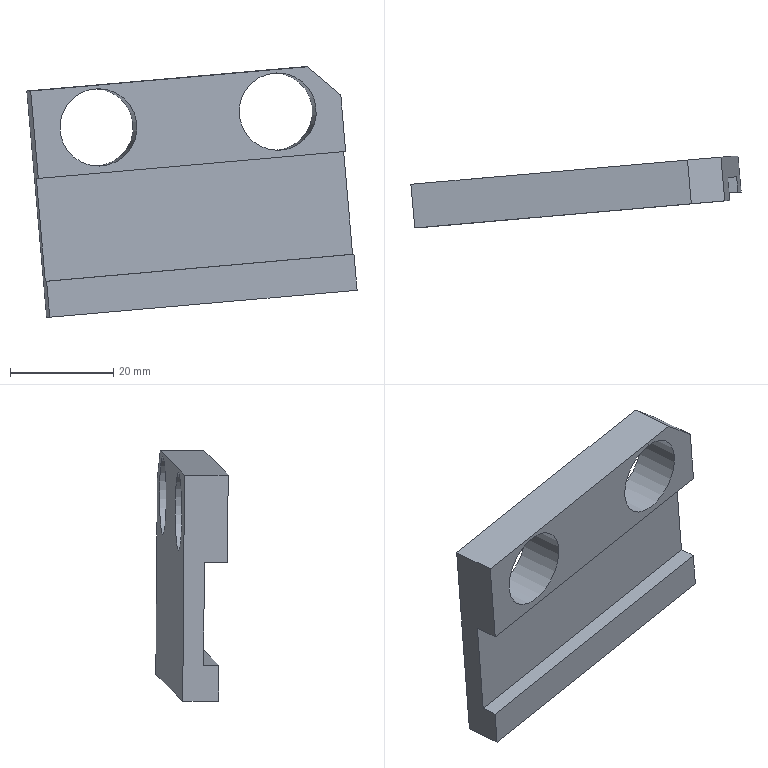Part | NX | features solid 2 | 1 solid | 13 faces | box 63.975 x 14.011 x 48.539 mm | volume 13253 mm3 | plane 11 | cylinder 2 | commonest cylinder face diameters 15 x2
STEP:
#1=CARTESIAN_POINT('',(-431.511,36.53,151.87));
#2=VERTEX_POINT('',#1);
#3=CARTESIAN_POINT('',(-436.313,36.11,146.125));
#4=DIRECTION('',(-0.08716,0.9962,0.));
#5=DIRECTION('',(0.6403,0.05602,0.766));
#6=AXIS2_PLACEMENT_3D('',#3,#4,#5);
#7=CIRCLE('',#6,7.5);
#8=EDGE_CURVE('',#2,#2,#7,.F.);
#9=ORIENTED_EDGE('',*,*,#8,.T.);
#10=EDGE_LOOP('',(#9));
#11=FACE_BOUND('',#10,.T.);
#12=CARTESIAN_POINT('',(-449.432,34.962,153.171));
#13=VERTEX_POINT('',#12);
#14=CARTESIAN_POINT('',(-395.842,39.651,157.877));
#15=VERTEX_POINT('',#14);
#16=CARTESIAN_POINT('',(-433.107,36.391,154.604));
#17=DIRECTION('',(0.9924,0.08682,0.08716));
#18=VECTOR('',#17,1000.);
#19=LINE('',#16,#18);
#20=EDGE_CURVE('',#13,#15,#19,.T.);
#21=ORIENTED_EDGE('',*,*,#20,.T.);
#22=CARTESIAN_POINT('',(-389.367,40.217,152.423));
#23=VERTEX_POINT('',#22);
#24=CARTESIAN_POINT('',(-394.52,39.767,156.764));
#25=DIRECTION('',(-0.7631,-0.06677,0.6428));
#26=VECTOR('',#25,1000.);
#27=LINE('',#24,#26);
#28=EDGE_CURVE('',#15,#23,#27,.F.);
#29=ORIENTED_EDGE('',*,*,#28,.T.);
#30=CARTESIAN_POINT('',(-386.068,40.506,114.567));
#31=VERTEX_POINT('',#30);
#32=CARTESIAN_POINT('',(-389.888,40.172,158.4));
#33=DIRECTION('',(0.08682,0.007596,-0.9962));
#34=VECTOR('',#33,1000.);
#35=LINE('',#32,#34);
#36=EDGE_CURVE('',#23,#31,#35,.T.);
#37=ORIENTED_EDGE('',*,*,#36,.T.);
#38=CARTESIAN_POINT('',(-445.612,35.297,109.338));
#39=VERTEX_POINT('',#38);
#40=CARTESIAN_POINT('',(-429.287,36.725,110.772));
#41=DIRECTION('',(0.9924,0.08682,0.08716));
#42=VECTOR('',#41,1000.);
#43=LINE('',#40,#42);
#44=EDGE_CURVE('',#39,#31,#43,.T.);
#45=ORIENTED_EDGE('',*,*,#44,.F.);
#46=CARTESIAN_POINT('',(-449.432,34.962,153.171));
#47=DIRECTION('',(0.08682,0.007596,-0.9962));
#48=VECTOR('',#47,1000.);
#49=LINE('',#46,#48);
#50=EDGE_CURVE('',#13,#39,#49,.T.);
#51=ORIENTED_EDGE('',*,*,#50,.F.);
#52=EDGE_LOOP('',(#21,#29,#37,#45,#51));
#53=FACE_BOUND('',#52,.T.);
#54=CARTESIAN_POINT('',(-396.777,39.569,154.92));
#55=VERTEX_POINT('',#54);
#56=CARTESIAN_POINT('',(-401.579,39.149,149.175));
#57=DIRECTION('',(-0.08716,0.9962,0.));
#58=DIRECTION('',(0.6403,0.05602,0.766));
#59=AXIS2_PLACEMENT_3D('',#56,#57,#58);
#60=CIRCLE('',#59,7.5);
#61=EDGE_CURVE('',#55,#55,#60,.F.);
#62=ORIENTED_EDGE('',*,*,#61,.T.);
#63=EDGE_LOOP('',(#62));
#64=FACE_BOUND('',#63,.T.);
#65=CARTESIAN_POINT('',(-393.411,39.864,158.091));
#66=DIRECTION('',(-0.08716,0.9962,0.));
#67=DIRECTION('',(-0.6403,-0.05602,-0.766));
#68=AXIS2_PLACEMENT_3D('',#65,#66,#67);
#69=PLANE('',#68);
#70=ADVANCED_FACE('',(#11,#53,#64),#69,.T.);
#71=CARTESIAN_POINT('',(-430.77,28.063,151.87));
#72=VERTEX_POINT('',#71);
#73=CARTESIAN_POINT('',(-435.572,27.643,146.125));
#74=DIRECTION('',(-0.08716,0.9962,0.));
#75=DIRECTION('',(0.6403,0.05602,0.766));
#76=AXIS2_PLACEMENT_3D('',#73,#74,#75);
#77=CIRCLE('',#76,7.5);
#78=EDGE_CURVE('',#72,#72,#77,.F.);
#79=ORIENTED_EDGE('',*,*,#78,.F.);
#80=EDGE_LOOP('',(#79));
#81=FACE_BOUND('',#80,.T.);
#82=CARTESIAN_POINT('',(-387.671,31.833,141.465));
#83=VERTEX_POINT('',#82);
#84=CARTESIAN_POINT('',(-388.626,31.75,152.423));
#85=VERTEX_POINT('',#84);
#86=CARTESIAN_POINT('',(-389.147,31.704,158.4));
#87=DIRECTION('',(0.08682,0.007596,-0.9962));
#88=VECTOR('',#87,1000.);
#89=LINE('',#86,#88);
#90=EDGE_CURVE('',#83,#85,#89,.F.);
#91=ORIENTED_EDGE('',*,*,#90,.T.);
#92=CARTESIAN_POINT('',(-395.102,31.183,157.877));
#93=VERTEX_POINT('',#92);
#94=CARTESIAN_POINT('',(-415.364,29.411,174.944));
#95=DIRECTION('',(-0.7631,-0.06677,0.6428));
#96=VECTOR('',#95,1000.);
#97=LINE('',#94,#96);
#98=EDGE_CURVE('',#85,#93,#97,.T.);
#99=ORIENTED_EDGE('',*,*,#98,.T.);
#100=CARTESIAN_POINT('',(-448.691,26.495,153.171));
#101=VERTEX_POINT('',#100);
#102=CARTESIAN_POINT('',(-432.366,27.923,154.604));
#103=DIRECTION('',(0.9924,0.08682,0.08716));
#104=VECTOR('',#103,1000.);
#105=LINE('',#102,#104);
#106=EDGE_CURVE('',#101,#93,#105,.T.);
#107=ORIENTED_EDGE('',*,*,#106,.F.);
#108=CARTESIAN_POINT('',(-447.215,26.624,136.235));
#109=VERTEX_POINT('',#108);
#110=CARTESIAN_POINT('',(-448.691,26.495,153.171));
#111=DIRECTION('',(-0.08682,-0.007596,0.9962));
#112=VECTOR('',#111,1000.);
#113=LINE('',#110,#112);
#114=EDGE_CURVE('',#109,#101,#113,.T.);
#115=ORIENTED_EDGE('',*,*,#114,.F.);
#116=CARTESIAN_POINT('',(-430.89,28.052,137.669));
#117=DIRECTION('',(0.9924,0.08682,0.08716));
#118=VECTOR('',#117,1000.);
#119=LINE('',#116,#118);
#120=EDGE_CURVE('',#109,#83,#119,.T.);
#121=ORIENTED_EDGE('',*,*,#120,.T.);
#122=EDGE_LOOP('',(#91,#99,#107,#115,#121));
#123=FACE_BOUND('',#122,.T.);
#124=CARTESIAN_POINT('',(-396.036,31.102,154.92));
#125=VERTEX_POINT('',#124);
#126=CARTESIAN_POINT('',(-400.838,30.681,149.175));
#127=DIRECTION('',(-0.08716,0.9962,0.));
#128=DIRECTION('',(0.6403,0.05602,0.766));
#129=AXIS2_PLACEMENT_3D('',#126,#127,#128);
#130=CIRCLE('',#129,7.5);
#131=EDGE_CURVE('',#125,#125,#130,.F.);
#132=ORIENTED_EDGE('',*,*,#131,.F.);
#133=EDGE_LOOP('',(#132));
#134=FACE_BOUND('',#133,.T.);
#135=CARTESIAN_POINT('',(-432.366,27.923,154.604));
#136=DIRECTION('',(-0.08716,0.9962,0.));
#137=DIRECTION('',(0.9924,0.08682,0.08716));
#138=AXIS2_PLACEMENT_3D('',#135,#136,#137);
#139=PLANE('',#138);
#140=ADVANCED_FACE('',(#81,#123,#134),#139,.F.);
#141=CARTESIAN_POINT('',(-447.608,31.107,136.235));
#142=VERTEX_POINT('',#141);
#143=CARTESIAN_POINT('',(-388.063,36.316,141.465));
#144=VERTEX_POINT('',#143);
#145=CARTESIAN_POINT('',(-391.586,36.008,141.155));
#146=DIRECTION('',(0.9924,0.08682,0.08716));
#147=VECTOR('',#146,1000.);
#148=LINE('',#145,#147);
#149=EDGE_CURVE('',#142,#144,#148,.T.);
#150=ORIENTED_EDGE('',*,*,#149,.F.);
#151=CARTESIAN_POINT('',(-445.871,31.259,116.312));
#152=VERTEX_POINT('',#151);
#153=CARTESIAN_POINT('',(-449.084,30.978,153.171));
#154=DIRECTION('',(0.08682,0.007596,-0.9962));
#155=VECTOR('',#154,1000.);
#156=LINE('',#153,#155);
#157=EDGE_CURVE('',#142,#152,#156,.T.);
#158=ORIENTED_EDGE('',*,*,#157,.T.);
#159=CARTESIAN_POINT('',(-386.327,36.468,121.541));
#160=VERTEX_POINT('',#159);
#161=CARTESIAN_POINT('',(-389.85,36.16,121.231));
#162=DIRECTION('',(0.9924,0.08682,0.08716));
#163=VECTOR('',#162,1000.);
#164=LINE('',#161,#163);
#165=EDGE_CURVE('',#152,#160,#164,.T.);
#166=ORIENTED_EDGE('',*,*,#165,.T.);
#167=CARTESIAN_POINT('',(-389.539,36.187,158.4));
#168=DIRECTION('',(0.08682,0.007596,-0.9962));
#169=VECTOR('',#168,1000.);
#170=LINE('',#167,#169);
#171=EDGE_CURVE('',#144,#160,#170,.T.);
#172=ORIENTED_EDGE('',*,*,#171,.F.);
#173=EDGE_LOOP('',(#150,#158,#166,#172));
#174=FACE_BOUND('',#173,.T.);
#175=CARTESIAN_POINT('',(-393.062,35.879,158.091));
#176=DIRECTION('',(-0.08716,0.9962,0.));
#177=DIRECTION('',(-0.6403,-0.05602,-0.766));
#178=AXIS2_PLACEMENT_3D('',#175,#176,#177);
#179=PLANE('',#178);
#180=ADVANCED_FACE('',(#174),#179,.F.);
#181=ORIENTED_EDGE('',*,*,#36,.F.);
#182=CARTESIAN_POINT('',(-389.018,36.233,152.423));
#183=DIRECTION('',(0.08716,-0.9962,0.));
#184=VECTOR('',#183,1000.);
#185=LINE('',#182,#184);
#186=EDGE_CURVE('',#23,#85,#185,.T.);
#187=ORIENTED_EDGE('',*,*,#186,.T.);
#188=ORIENTED_EDGE('',*,*,#90,.F.);
#189=CARTESIAN_POINT('',(-388.151,37.312,141.465));
#190=DIRECTION('',(0.08716,-0.9962,0.));
#191=VECTOR('',#190,1000.);
#192=LINE('',#189,#191);
#193=EDGE_CURVE('',#144,#83,#192,.T.);
#194=ORIENTED_EDGE('',*,*,#193,.F.);
#195=ORIENTED_EDGE('',*,*,#171,.T.);
#196=CARTESIAN_POINT('',(-386.065,33.48,121.541));
#197=VERTEX_POINT('',#196);
#198=CARTESIAN_POINT('',(-386.414,37.464,121.541));
#199=DIRECTION('',(0.08716,-0.9962,0.));
#200=VECTOR('',#199,1000.);
#201=LINE('',#198,#200);
#202=EDGE_CURVE('',#160,#197,#201,.T.);
#203=ORIENTED_EDGE('',*,*,#202,.T.);
#204=CARTESIAN_POINT('',(-385.458,33.533,114.567));
#205=VERTEX_POINT('',#204);
#206=CARTESIAN_POINT('',(-389.278,33.199,158.4));
#207=DIRECTION('',(0.08682,0.007596,-0.9962));
#208=VECTOR('',#207,1000.);
#209=LINE('',#206,#208);
#210=EDGE_CURVE('',#197,#205,#209,.T.);
#211=ORIENTED_EDGE('',*,*,#210,.T.);
#212=CARTESIAN_POINT('',(-385.719,36.521,114.567));
#213=DIRECTION('',(-0.08716,0.9962,0.));
#214=VECTOR('',#213,1000.);
#215=LINE('',#212,#214);
#216=EDGE_CURVE('',#205,#31,#215,.T.);
#217=ORIENTED_EDGE('',*,*,#216,.T.);
#218=EDGE_LOOP('',(#181,#187,#188,#194,#195,#203,#211,#217));
#219=FACE_BOUND('',#218,.T.);
#220=CARTESIAN_POINT('',(-389.539,36.187,158.4));
#221=DIRECTION('',(-0.9924,-0.08682,-0.08716));
#222=DIRECTION('',(-0.08682,-0.007596,0.9962));
#223=AXIS2_PLACEMENT_3D('',#220,#221,#222);
#224=PLANE('',#223);
#225=ADVANCED_FACE('',(#219),#224,.F.);
#226=CARTESIAN_POINT('',(-445.002,28.323,109.338));
#227=VERTEX_POINT('',#226);
#228=CARTESIAN_POINT('',(-428.677,29.752,110.772));
#229=DIRECTION('',(0.9924,0.08682,0.08716));
#230=VECTOR('',#229,1000.);
#231=LINE('',#228,#230);
#232=EDGE_CURVE('',#227,#205,#231,.T.);
#233=ORIENTED_EDGE('',*,*,#232,.F.);
#234=CARTESIAN_POINT('',(-445.263,31.312,109.338));
#235=DIRECTION('',(-0.08716,0.9962,0.));
#236=VECTOR('',#235,1000.);
#237=LINE('',#234,#236);
#238=EDGE_CURVE('',#227,#39,#237,.T.);
#239=ORIENTED_EDGE('',*,*,#238,.T.);
#240=ORIENTED_EDGE('',*,*,#44,.T.);
#241=ORIENTED_EDGE('',*,*,#216,.F.);
#242=EDGE_LOOP('',(#233,#239,#240,#241));
#243=FACE_BOUND('',#242,.T.);
#244=CARTESIAN_POINT('',(-428.938,32.74,110.772));
#245=DIRECTION('',(0.08682,0.007596,-0.9962));
#246=DIRECTION('',(-0.9924,-0.08682,-0.08716));
#247=AXIS2_PLACEMENT_3D('',#244,#245,#246);
#248=PLANE('',#247);
#249=ADVANCED_FACE('',(#243),#248,.T.);
#250=ORIENTED_EDGE('',*,*,#106,.T.);
#251=CARTESIAN_POINT('',(-395.494,35.666,157.877));
#252=DIRECTION('',(-0.08716,0.9962,0.));
#253=VECTOR('',#252,1000.);
#254=LINE('',#251,#253);
#255=EDGE_CURVE('',#93,#15,#254,.T.);
#256=ORIENTED_EDGE('',*,*,#255,.T.);
#257=ORIENTED_EDGE('',*,*,#20,.F.);
#258=CARTESIAN_POINT('',(-449.084,30.978,153.171));
#259=DIRECTION('',(-0.08716,0.9962,0.));
#260=VECTOR('',#259,1000.);
#261=LINE('',#258,#260);
#262=EDGE_CURVE('',#101,#13,#261,.T.);
#263=ORIENTED_EDGE('',*,*,#262,.F.);
#264=EDGE_LOOP('',(#250,#256,#257,#263));
#265=FACE_BOUND('',#264,.T.);
#266=CARTESIAN_POINT('',(-432.759,32.406,154.604));
#267=DIRECTION('',(0.08682,0.007596,-0.9962));
#268=DIRECTION('',(-0.9924,-0.08682,-0.08716));
#269=AXIS2_PLACEMENT_3D('',#266,#267,#268);
#270=PLANE('',#269);
#271=ADVANCED_FACE('',(#265),#270,.F.);
#272=ORIENTED_EDGE('',*,*,#120,.F.);
#273=CARTESIAN_POINT('',(-447.695,32.103,136.235));
#274=DIRECTION('',(0.08716,-0.9962,0.));
#275=VECTOR('',#274,1000.);
#276=LINE('',#273,#275);
#277=EDGE_CURVE('',#142,#109,#276,.T.);
#278=ORIENTED_EDGE('',*,*,#277,.F.);
#279=ORIENTED_EDGE('',*,*,#149,.T.);
#280=ORIENTED_EDGE('',*,*,#193,.T.);
#281=EDGE_LOOP('',(#272,#278,#279,#280));
#282=FACE_BOUND('',#281,.T.);
#283=CARTESIAN_POINT('',(-431.37,33.531,137.669));
#284=DIRECTION('',(-0.08682,-0.007596,0.9962));
#285=DIRECTION('',(0.9924,0.08682,0.08716));
#286=AXIS2_PLACEMENT_3D('',#283,#284,#285);
#287=PLANE('',#286);
#288=ADVANCED_FACE('',(#282),#287,.F.);
#289=ORIENTED_EDGE('',*,*,#165,.F.);
#290=CARTESIAN_POINT('',(-445.61,28.27,116.312));
#291=VERTEX_POINT('',#290);
#292=CARTESIAN_POINT('',(-445.958,32.255,116.312));
#293=DIRECTION('',(0.08716,-0.9962,0.));
#294=VECTOR('',#293,1000.);
#295=LINE('',#292,#294);
#296=EDGE_CURVE('',#152,#291,#295,.T.);
#297=ORIENTED_EDGE('',*,*,#296,.T.);
#298=CARTESIAN_POINT('',(-429.285,29.698,117.745));
#299=DIRECTION('',(0.9924,0.08682,0.08716));
#300=VECTOR('',#299,1000.);
#301=LINE('',#298,#300);
#302=EDGE_CURVE('',#291,#197,#301,.T.);
#303=ORIENTED_EDGE('',*,*,#302,.T.);
#304=ORIENTED_EDGE('',*,*,#202,.F.);
#305=EDGE_LOOP('',(#289,#297,#303,#304));
#306=FACE_BOUND('',#305,.T.);
#307=CARTESIAN_POINT('',(-429.633,33.683,117.745));
#308=DIRECTION('',(-0.08682,-0.007596,0.9962));
#309=DIRECTION('',(0.9924,0.08682,0.08716));
#310=AXIS2_PLACEMENT_3D('',#307,#308,#309);
#311=PLANE('',#310);
#312=ADVANCED_FACE('',(#306),#311,.T.);
#313=ORIENTED_EDGE('',*,*,#210,.F.);
#314=ORIENTED_EDGE('',*,*,#302,.F.);
#315=CARTESIAN_POINT('',(-445.002,28.323,109.338));
#316=DIRECTION('',(-0.08682,-0.007596,0.9962));
#317=VECTOR('',#316,1000.);
#318=LINE('',#315,#317);
#319=EDGE_CURVE('',#291,#227,#318,.F.);
#320=ORIENTED_EDGE('',*,*,#319,.T.);
#321=ORIENTED_EDGE('',*,*,#232,.T.);
#322=EDGE_LOOP('',(#313,#314,#320,#321));
#323=FACE_BOUND('',#322,.T.);
#324=CARTESIAN_POINT('',(-428.677,29.752,110.772));
#325=DIRECTION('',(-0.08716,0.9962,0.));
#326=DIRECTION('',(0.9924,0.08682,0.08716));
#327=AXIS2_PLACEMENT_3D('',#324,#325,#326);
#328=PLANE('',#327);
#329=ADVANCED_FACE('',(#323),#328,.F.);
#330=ORIENTED_EDGE('',*,*,#50,.T.);
#331=ORIENTED_EDGE('',*,*,#238,.F.);
#332=ORIENTED_EDGE('',*,*,#319,.F.);
#333=ORIENTED_EDGE('',*,*,#296,.F.);
#334=ORIENTED_EDGE('',*,*,#157,.F.);
#335=ORIENTED_EDGE('',*,*,#277,.T.);
#336=ORIENTED_EDGE('',*,*,#114,.T.);
#337=ORIENTED_EDGE('',*,*,#262,.T.);
#338=EDGE_LOOP('',(#330,#331,#332,#333,#334,#335,#336,#337));
#339=FACE_BOUND('',#338,.T.);
#340=CARTESIAN_POINT('',(-449.084,30.978,153.171));
#341=DIRECTION('',(-0.9924,-0.08682,-0.08716));
#342=DIRECTION('',(-0.08682,-0.007596,0.9962));
#343=AXIS2_PLACEMENT_3D('',#340,#341,#342);
#344=PLANE('',#343);
#345=ADVANCED_FACE('',(#339),#344,.T.);
#346=ORIENTED_EDGE('',*,*,#78,.T.);
#347=EDGE_LOOP('',(#346));
#348=FACE_BOUND('',#347,.T.);
#349=ORIENTED_EDGE('',*,*,#8,.F.);
#350=EDGE_LOOP('',(#349));
#351=FACE_BOUND('',#350,.T.);
#352=CARTESIAN_POINT('',(-435.572,27.643,146.125));
#353=DIRECTION('',(-0.08716,0.9962,0.));
#354=DIRECTION('',(0.6403,0.05602,0.766));
#355=AXIS2_PLACEMENT_3D('',#352,#353,#354);
#356=CYLINDRICAL_SURFACE('',#355,7.5);
#357=ADVANCED_FACE('',(#348,#351),#356,.F.);
#358=ORIENTED_EDGE('',*,*,#131,.T.);
#359=EDGE_LOOP('',(#358));
#360=FACE_BOUND('',#359,.T.);
#361=ORIENTED_EDGE('',*,*,#61,.F.);
#362=EDGE_LOOP('',(#361));
#363=FACE_BOUND('',#362,.T.);
#364=CARTESIAN_POINT('',(-400.838,30.681,149.175));
#365=DIRECTION('',(-0.08716,0.9962,0.));
#366=DIRECTION('',(0.6403,0.05602,0.766));
#367=AXIS2_PLACEMENT_3D('',#364,#365,#366);
#368=CYLINDRICAL_SURFACE('',#367,7.5);
#369=ADVANCED_FACE('',(#360,#363),#368,.F.);
#370=ORIENTED_EDGE('',*,*,#98,.F.);
#371=ORIENTED_EDGE('',*,*,#186,.F.);
#372=ORIENTED_EDGE('',*,*,#28,.F.);
#373=ORIENTED_EDGE('',*,*,#255,.F.);
#374=EDGE_LOOP('',(#370,#371,#372,#373));
#375=FACE_BOUND('',#374,.T.);
#376=CARTESIAN_POINT('',(-395.494,35.666,157.877));
#377=DIRECTION('',(-0.6403,-0.05602,-0.766));
#378=DIRECTION('',(-0.7631,-0.06677,0.6428));
#379=AXIS2_PLACEMENT_3D('',#376,#377,#378);
#380=PLANE('',#379);
#381=ADVANCED_FACE('',(#375),#380,.F.);
#382=CLOSED_SHELL('',(#70,#140,#180,#225,#249,#271,#288,#312,#329,#345,#357,#369,#381));
#383=MANIFOLD_SOLID_BREP('',#382);
#384=(LENGTH_UNIT()NAMED_UNIT(*)SI_UNIT(.MILLI.,.METRE.));
#385=UNCERTAINTY_MEASURE_WITH_UNIT(LENGTH_MEASURE(0.00001),#384,'','');
#386=(NAMED_UNIT(*)PLANE_ANGLE_UNIT()SI_UNIT($,.RADIAN.));
#387=(NAMED_UNIT(*)SI_UNIT($,.STERADIAN.)SOLID_ANGLE_UNIT());
#388=(GEOMETRIC_REPRESENTATION_CONTEXT(3)GLOBAL_UNCERTAINTY_ASSIGNED_CONTEXT((#385))GLOBAL_UNIT_ASSIGNED_CONTEXT((#384,#386,#387))REPRESENTATION_CONTEXT('',''));
#389=ADVANCED_BREP_SHAPE_REPRESENTATION('',(#383),#388);